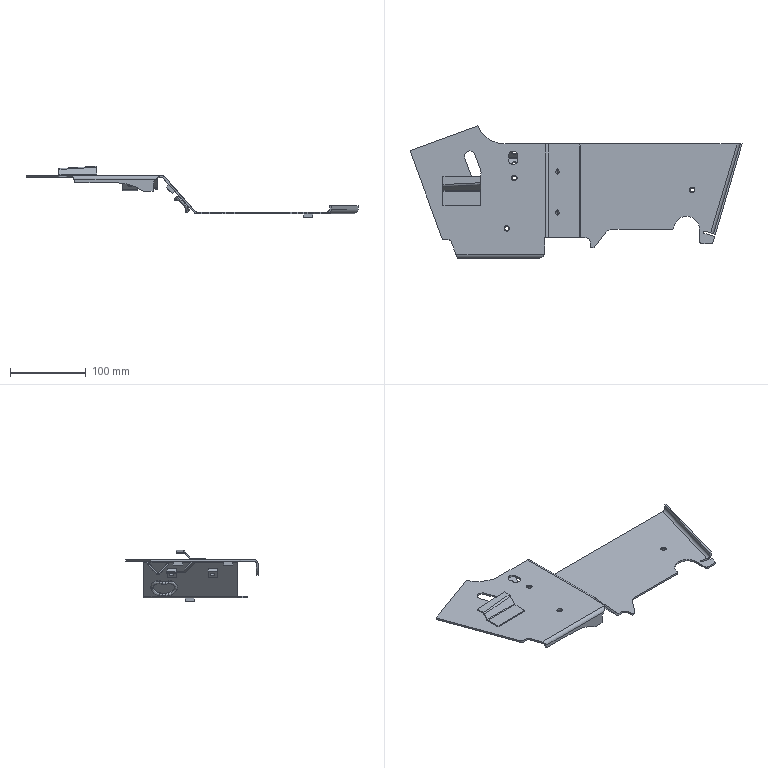Part | SolidWorks | features CompositeCurve 2 | 10 solids | 235 faces | box 437.3 x 174 x 67.601 mm | volume 137259 mm3 | plane 138 | cylinder 78 | spline 19 | commonest cylinder face diameters 5 x13 7.2 x10 4 x8 3.2 x4 6 x4 6.4 x4